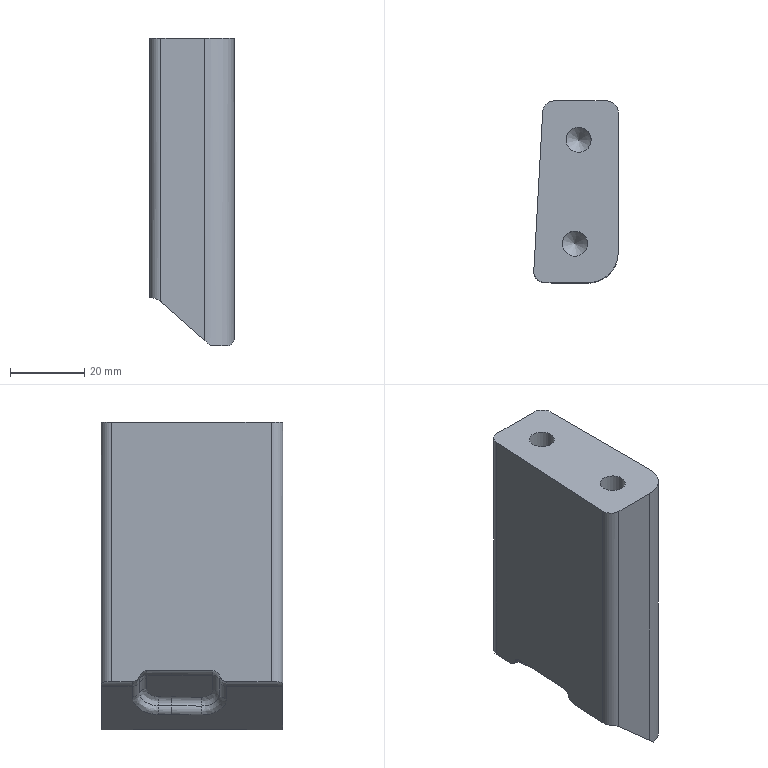Part | NX | features solid 2 | 1 solid | 45 faces | box 22.763 x 49 x 83 mm | volume 77399 mm3 | cylinder 21 | spline 12 | plane 10 | cone 2 | commonest cylinder face diameters 4 x11 10 x4 6 x3 6.8 x2 16 x1